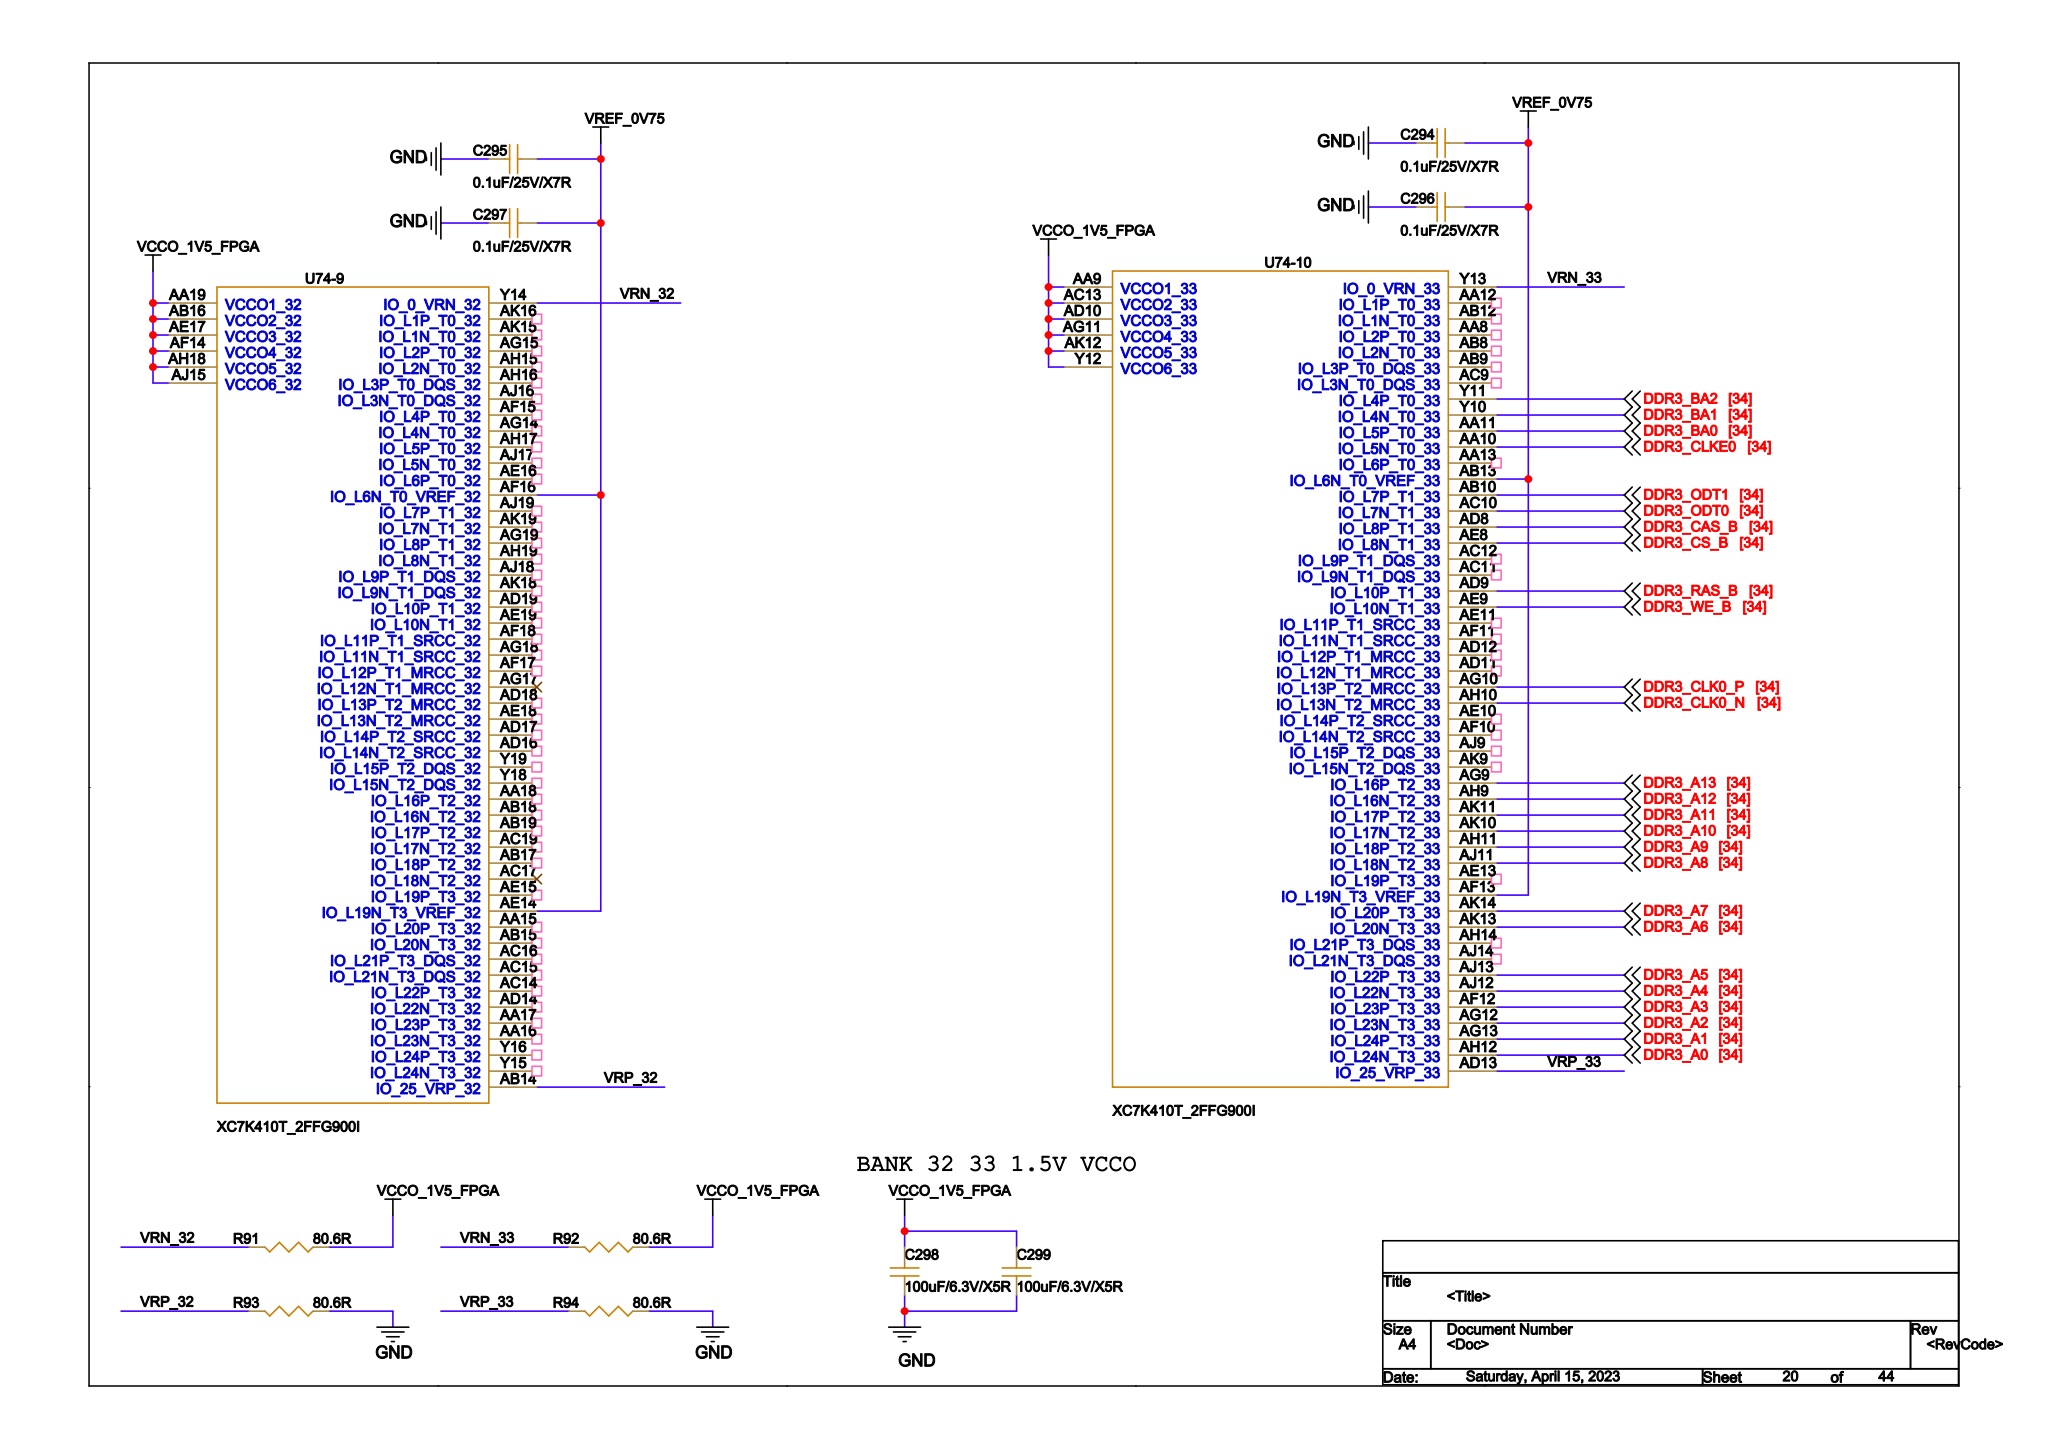Circuit board | Cadence Allegro | 1034 parts | 912 nets | one sheet of the schematic
Parts on this sheet (reference | value | footprint):
C294 | 0.1uF/25V/X7R | C0402_BGA
C295 | 0.1uF/25V/X7R | C0402_BGA
C296 | 0.1uF/25V/X7R | C0402_BGA
C297 | 0.1uF/25V/X7R | C0402_BGA
C298 | 100uF/6.3V/X5R | C0402_BGA
C299 | 100uF/6.3V/X5R | C0402_BGA
R91 | 80.6R | R0402
R92 | 80.6R | R0402
R93 | 80.6R | R0402
R94 | 80.6R | R0402
Nets of these parts (net: part-pin ...):
GND: C294-2 C295-2 C296-2 C297-2 C298-1 C299-1 R93-1 R94-1
VCCO_1V5_FPGA: C298-2 C299-2 R91-1 R92-1
VREF_0V75: C294-1 C295-1 C296-1 C297-1
VRN_32: R91-2
VRN_33: R92-2
VRP_32: R93-2
VRP_33: R94-2